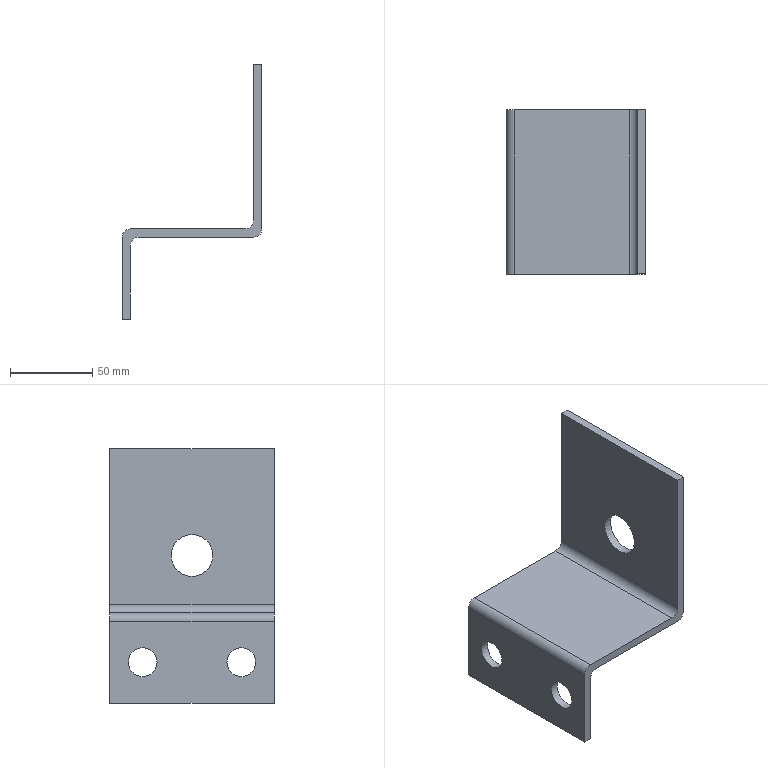Part | NX | features solid 2 | 1 solid | 17 faces | box 85 x 100 x 155 mm | volume 112541 mm3 | plane 10 | cylinder 7 | commonest cylinder face diameters 10 x4 17.5 x2 25.5 x1
STEP:
#1=CARTESIAN_POINT('',(-1095.,-291.25,-600.));
#2=VERTEX_POINT('',#1);
#3=CARTESIAN_POINT('',(-1095.,-300.,-600.));
#4=DIRECTION('',(1.,0.,0.));
#5=DIRECTION('',(0.,1.,0.));
#6=AXIS2_PLACEMENT_3D('',#3,#4,#5);
#7=CIRCLE('',#6,8.75);
#8=EDGE_CURVE('',#2,#2,#7,.T.);
#9=ORIENTED_EDGE('',*,*,#8,.F.);
#10=EDGE_LOOP('',(#9));
#11=FACE_BOUND('',#10,.T.);
#12=CARTESIAN_POINT('',(-1095.,-231.25,-600.));
#13=VERTEX_POINT('',#12);
#14=CARTESIAN_POINT('',(-1095.,-240.,-600.));
#15=DIRECTION('',(1.,0.,0.));
#16=DIRECTION('',(0.,1.,0.));
#17=AXIS2_PLACEMENT_3D('',#14,#15,#16);
#18=CIRCLE('',#17,8.75);
#19=EDGE_CURVE('',#13,#13,#18,.T.);
#20=ORIENTED_EDGE('',*,*,#19,.F.);
#21=EDGE_LOOP('',(#20));
#22=FACE_BOUND('',#21,.T.);
#23=CARTESIAN_POINT('',(-1095.,-220.,-580.));
#24=VERTEX_POINT('',#23);
#25=CARTESIAN_POINT('',(-1095.,-220.,-625.));
#26=VERTEX_POINT('',#25);
#27=CARTESIAN_POINT('',(-1095.,-220.,-570.));
#28=DIRECTION('',(0.,0.,1.));
#29=VECTOR('',#28,1000.);
#30=LINE('',#27,#29);
#31=EDGE_CURVE('',#24,#26,#30,.F.);
#32=ORIENTED_EDGE('',*,*,#31,.F.);
#33=CARTESIAN_POINT('',(-1095.,-320.,-580.));
#34=VERTEX_POINT('',#33);
#35=CARTESIAN_POINT('',(-1095.,-220.,-580.));
#36=DIRECTION('',(0.,-1.,0.));
#37=VECTOR('',#36,1000.);
#38=LINE('',#35,#37);
#39=EDGE_CURVE('',#24,#34,#38,.T.);
#40=ORIENTED_EDGE('',*,*,#39,.T.);
#41=CARTESIAN_POINT('',(-1095.,-320.,-625.));
#42=VERTEX_POINT('',#41);
#43=CARTESIAN_POINT('',(-1095.,-320.,-570.));
#44=DIRECTION('',(0.,0.,1.));
#45=VECTOR('',#44,1000.);
#46=LINE('',#43,#45);
#47=EDGE_CURVE('',#34,#42,#46,.F.);
#48=ORIENTED_EDGE('',*,*,#47,.T.);
#49=CARTESIAN_POINT('',(-1095.,-220.,-625.));
#50=DIRECTION('',(0.,1.,0.));
#51=VECTOR('',#50,1000.);
#52=LINE('',#49,#51);
#53=EDGE_CURVE('',#26,#42,#52,.F.);
#54=ORIENTED_EDGE('',*,*,#53,.F.);
#55=EDGE_LOOP('',(#32,#40,#48,#54));
#56=FACE_BOUND('',#55,.T.);
#57=CARTESIAN_POINT('',(-1095.,-220.,-570.));
#58=DIRECTION('',(1.,0.,0.));
#59=DIRECTION('',(0.,1.,0.));
#60=AXIS2_PLACEMENT_3D('',#57,#58,#59);
#61=PLANE('',#60);
#62=ADVANCED_FACE('',(#11,#22,#56),#61,.T.);
#63=CARTESIAN_POINT('',(-1095.,-220.,-570.));
#64=VERTEX_POINT('',#63);
#65=CARTESIAN_POINT('',(-1025.,-220.,-570.));
#66=VERTEX_POINT('',#65);
#67=CARTESIAN_POINT('',(-1100.,-220.,-570.));
#68=DIRECTION('',(1.,0.,0.));
#69=VECTOR('',#68,1000.);
#70=LINE('',#67,#69);
#71=EDGE_CURVE('',#64,#66,#70,.T.);
#72=ORIENTED_EDGE('',*,*,#71,.F.);
#73=CARTESIAN_POINT('',(-1095.,-320.,-570.));
#74=VERTEX_POINT('',#73);
#75=CARTESIAN_POINT('',(-1095.,-320.,-570.));
#76=DIRECTION('',(0.,-1.,0.));
#77=VECTOR('',#76,1000.);
#78=LINE('',#75,#77);
#79=EDGE_CURVE('',#64,#74,#78,.T.);
#80=ORIENTED_EDGE('',*,*,#79,.T.);
#81=CARTESIAN_POINT('',(-1025.,-320.,-570.));
#82=VERTEX_POINT('',#81);
#83=CARTESIAN_POINT('',(-1100.,-320.,-570.));
#84=DIRECTION('',(1.,0.,0.));
#85=VECTOR('',#84,1000.);
#86=LINE('',#83,#85);
#87=EDGE_CURVE('',#74,#82,#86,.T.);
#88=ORIENTED_EDGE('',*,*,#87,.T.);
#89=CARTESIAN_POINT('',(-1025.,-220.,-570.));
#90=DIRECTION('',(0.,-1.,0.));
#91=VECTOR('',#90,1000.);
#92=LINE('',#89,#91);
#93=EDGE_CURVE('',#82,#66,#92,.F.);
#94=ORIENTED_EDGE('',*,*,#93,.T.);
#95=EDGE_LOOP('',(#72,#80,#88,#94));
#96=FACE_BOUND('',#95,.T.);
#97=CARTESIAN_POINT('',(-1100.,-220.,-570.));
#98=DIRECTION('',(0.,0.,1.));
#99=DIRECTION('',(0.,-1.,0.));
#100=AXIS2_PLACEMENT_3D('',#97,#98,#99);
#101=PLANE('',#100);
#102=ADVANCED_FACE('',(#96),#101,.T.);
#103=ORIENTED_EDGE('',*,*,#87,.F.);
#104=CARTESIAN_POINT('',(-1100.,-320.,-575.));
#105=VERTEX_POINT('',#104);
#106=CARTESIAN_POINT('',(-1095.,-320.,-575.));
#107=DIRECTION('',(0.,-1.,0.));
#108=DIRECTION('',(1.,0.,0.));
#109=AXIS2_PLACEMENT_3D('',#106,#107,#108);
#110=CIRCLE('',#109,5.);
#111=EDGE_CURVE('',#74,#105,#110,.T.);
#112=ORIENTED_EDGE('',*,*,#111,.T.);
#113=CARTESIAN_POINT('',(-1100.,-320.,-625.));
#114=VERTEX_POINT('',#113);
#115=CARTESIAN_POINT('',(-1100.,-320.,-570.));
#116=DIRECTION('',(0.,0.,-1.));
#117=VECTOR('',#116,1000.);
#118=LINE('',#115,#117);
#119=EDGE_CURVE('',#105,#114,#118,.T.);
#120=ORIENTED_EDGE('',*,*,#119,.T.);
#121=CARTESIAN_POINT('',(-1100.,-320.,-625.));
#122=DIRECTION('',(-1.,0.,0.));
#123=VECTOR('',#122,1000.);
#124=LINE('',#121,#123);
#125=EDGE_CURVE('',#114,#42,#124,.F.);
#126=ORIENTED_EDGE('',*,*,#125,.T.);
#127=ORIENTED_EDGE('',*,*,#47,.F.);
#128=CARTESIAN_POINT('',(-1090.,-320.,-575.));
#129=VERTEX_POINT('',#128);
#130=CARTESIAN_POINT('',(-1090.,-320.,-580.));
#131=DIRECTION('',(0.,-1.,0.));
#132=DIRECTION('',(1.,0.,0.));
#133=AXIS2_PLACEMENT_3D('',#130,#131,#132);
#134=CIRCLE('',#133,5.);
#135=EDGE_CURVE('',#34,#129,#134,.F.);
#136=ORIENTED_EDGE('',*,*,#135,.T.);
#137=CARTESIAN_POINT('',(-1020.,-320.,-575.));
#138=VERTEX_POINT('',#137);
#139=CARTESIAN_POINT('',(-1015.,-320.,-575.));
#140=DIRECTION('',(-1.,0.,0.));
#141=VECTOR('',#140,1000.);
#142=LINE('',#139,#141);
#143=EDGE_CURVE('',#138,#129,#142,.T.);
#144=ORIENTED_EDGE('',*,*,#143,.F.);
#145=CARTESIAN_POINT('',(-1015.,-320.,-570.));
#146=VERTEX_POINT('',#145);
#147=CARTESIAN_POINT('',(-1020.,-320.,-570.));
#148=DIRECTION('',(0.,-1.,0.));
#149=DIRECTION('',(1.,0.,0.));
#150=AXIS2_PLACEMENT_3D('',#147,#148,#149);
#151=CIRCLE('',#150,5.);
#152=EDGE_CURVE('',#138,#146,#151,.T.);
#153=ORIENTED_EDGE('',*,*,#152,.T.);
#154=CARTESIAN_POINT('',(-1015.,-320.,-470.));
#155=VERTEX_POINT('',#154);
#156=CARTESIAN_POINT('',(-1015.,-320.,-575.));
#157=DIRECTION('',(0.,0.,1.));
#158=VECTOR('',#157,1000.);
#159=LINE('',#156,#158);
#160=EDGE_CURVE('',#146,#155,#159,.T.);
#161=ORIENTED_EDGE('',*,*,#160,.T.);
#162=CARTESIAN_POINT('',(-1020.,-320.,-470.));
#163=VERTEX_POINT('',#162);
#164=CARTESIAN_POINT('',(-1010.,-320.,-470.));
#165=DIRECTION('',(-1.,0.,0.));
#166=VECTOR('',#165,1000.);
#167=LINE('',#164,#166);
#168=EDGE_CURVE('',#155,#163,#167,.T.);
#169=ORIENTED_EDGE('',*,*,#168,.T.);
#170=CARTESIAN_POINT('',(-1020.,-320.,-565.));
#171=VERTEX_POINT('',#170);
#172=CARTESIAN_POINT('',(-1020.,-320.,-575.));
#173=DIRECTION('',(0.,0.,1.));
#174=VECTOR('',#173,1000.);
#175=LINE('',#172,#174);
#176=EDGE_CURVE('',#171,#163,#175,.T.);
#177=ORIENTED_EDGE('',*,*,#176,.F.);
#178=CARTESIAN_POINT('',(-1025.,-320.,-565.));
#179=DIRECTION('',(0.,-1.,0.));
#180=DIRECTION('',(1.,0.,0.));
#181=AXIS2_PLACEMENT_3D('',#178,#179,#180);
#182=CIRCLE('',#181,5.);
#183=EDGE_CURVE('',#171,#82,#182,.F.);
#184=ORIENTED_EDGE('',*,*,#183,.T.);
#185=EDGE_LOOP('',(#103,#112,#120,#126,#127,#136,#144,#153,#161,#169,#177,#184));
#186=FACE_BOUND('',#185,.T.);
#187=CARTESIAN_POINT('',(-1100.,-320.,-570.));
#188=DIRECTION('',(0.,-1.,0.));
#189=DIRECTION('',(0.,0.,-1.));
#190=AXIS2_PLACEMENT_3D('',#187,#188,#189);
#191=PLANE('',#190);
#192=ADVANCED_FACE('',(#186),#191,.T.);
#193=ORIENTED_EDGE('',*,*,#125,.F.);
#194=CARTESIAN_POINT('',(-1100.,-220.,-625.));
#195=VERTEX_POINT('',#194);
#196=CARTESIAN_POINT('',(-1100.,-220.,-625.));
#197=DIRECTION('',(0.,1.,0.));
#198=VECTOR('',#197,1000.);
#199=LINE('',#196,#198);
#200=EDGE_CURVE('',#195,#114,#199,.F.);
#201=ORIENTED_EDGE('',*,*,#200,.F.);
#202=CARTESIAN_POINT('',(-1100.,-220.,-625.));
#203=DIRECTION('',(1.,0.,0.));
#204=VECTOR('',#203,1000.);
#205=LINE('',#202,#204);
#206=EDGE_CURVE('',#195,#26,#205,.T.);
#207=ORIENTED_EDGE('',*,*,#206,.T.);
#208=ORIENTED_EDGE('',*,*,#53,.T.);
#209=EDGE_LOOP('',(#193,#201,#207,#208));
#210=FACE_BOUND('',#209,.T.);
#211=CARTESIAN_POINT('',(-1100.,-220.,-625.));
#212=DIRECTION('',(0.,0.,1.));
#213=DIRECTION('',(0.,-1.,0.));
#214=AXIS2_PLACEMENT_3D('',#211,#212,#213);
#215=PLANE('',#214);
#216=ADVANCED_FACE('',(#210),#215,.F.);
#217=CARTESIAN_POINT('',(-1100.,-220.,-575.));
#218=VERTEX_POINT('',#217);
#219=CARTESIAN_POINT('',(-1100.,-220.,-570.));
#220=DIRECTION('',(0.,0.,-1.));
#221=VECTOR('',#220,1000.);
#222=LINE('',#219,#221);
#223=EDGE_CURVE('',#218,#195,#222,.T.);
#224=ORIENTED_EDGE('',*,*,#223,.F.);
#225=CARTESIAN_POINT('',(-1095.,-220.,-575.));
#226=DIRECTION('',(0.,-1.,0.));
#227=DIRECTION('',(1.,0.,0.));
#228=AXIS2_PLACEMENT_3D('',#225,#226,#227);
#229=CIRCLE('',#228,5.);
#230=EDGE_CURVE('',#218,#64,#229,.F.);
#231=ORIENTED_EDGE('',*,*,#230,.T.);
#232=ORIENTED_EDGE('',*,*,#71,.T.);
#233=CARTESIAN_POINT('',(-1020.,-220.,-565.));
#234=VERTEX_POINT('',#233);
#235=CARTESIAN_POINT('',(-1025.,-220.,-565.));
#236=DIRECTION('',(0.,-1.,0.));
#237=DIRECTION('',(1.,0.,0.));
#238=AXIS2_PLACEMENT_3D('',#235,#236,#237);
#239=CIRCLE('',#238,5.);
#240=EDGE_CURVE('',#66,#234,#239,.T.);
#241=ORIENTED_EDGE('',*,*,#240,.T.);
#242=CARTESIAN_POINT('',(-1020.,-220.,-470.));
#243=VERTEX_POINT('',#242);
#244=CARTESIAN_POINT('',(-1020.,-220.,-570.));
#245=DIRECTION('',(0.,0.,-1.));
#246=VECTOR('',#245,1000.);
#247=LINE('',#244,#246);
#248=EDGE_CURVE('',#234,#243,#247,.F.);
#249=ORIENTED_EDGE('',*,*,#248,.T.);
#250=CARTESIAN_POINT('',(-1015.,-220.,-470.));
#251=VERTEX_POINT('',#250);
#252=CARTESIAN_POINT('',(-1015.,-220.,-470.));
#253=DIRECTION('',(1.,0.,0.));
#254=VECTOR('',#253,1000.);
#255=LINE('',#252,#254);
#256=EDGE_CURVE('',#251,#243,#255,.F.);
#257=ORIENTED_EDGE('',*,*,#256,.F.);
#258=CARTESIAN_POINT('',(-1015.,-220.,-570.));
#259=VERTEX_POINT('',#258);
#260=CARTESIAN_POINT('',(-1015.,-220.,-570.));
#261=DIRECTION('',(0.,0.,-1.));
#262=VECTOR('',#261,1000.);
#263=LINE('',#260,#262);
#264=EDGE_CURVE('',#259,#251,#263,.F.);
#265=ORIENTED_EDGE('',*,*,#264,.F.);
#266=CARTESIAN_POINT('',(-1020.,-220.,-575.));
#267=VERTEX_POINT('',#266);
#268=CARTESIAN_POINT('',(-1020.,-220.,-570.));
#269=DIRECTION('',(0.,-1.,0.));
#270=DIRECTION('',(1.,0.,0.));
#271=AXIS2_PLACEMENT_3D('',#268,#269,#270);
#272=CIRCLE('',#271,5.);
#273=EDGE_CURVE('',#259,#267,#272,.F.);
#274=ORIENTED_EDGE('',*,*,#273,.T.);
#275=CARTESIAN_POINT('',(-1090.,-220.,-575.));
#276=VERTEX_POINT('',#275);
#277=CARTESIAN_POINT('',(-1015.,-220.,-575.));
#278=DIRECTION('',(-1.,0.,0.));
#279=VECTOR('',#278,1000.);
#280=LINE('',#277,#279);
#281=EDGE_CURVE('',#267,#276,#280,.T.);
#282=ORIENTED_EDGE('',*,*,#281,.T.);
#283=CARTESIAN_POINT('',(-1090.,-220.,-580.));
#284=DIRECTION('',(0.,-1.,0.));
#285=DIRECTION('',(1.,0.,0.));
#286=AXIS2_PLACEMENT_3D('',#283,#284,#285);
#287=CIRCLE('',#286,5.);
#288=EDGE_CURVE('',#276,#24,#287,.T.);
#289=ORIENTED_EDGE('',*,*,#288,.T.);
#290=ORIENTED_EDGE('',*,*,#31,.T.);
#291=ORIENTED_EDGE('',*,*,#206,.F.);
#292=EDGE_LOOP('',(#224,#231,#232,#241,#249,#257,#265,#274,#282,#289,#290,#291));
#293=FACE_BOUND('',#292,.T.);
#294=CARTESIAN_POINT('',(-1100.,-220.,-570.));
#295=DIRECTION('',(0.,-1.,0.));
#296=DIRECTION('',(0.,0.,-1.));
#297=AXIS2_PLACEMENT_3D('',#294,#295,#296);
#298=PLANE('',#297);
#299=ADVANCED_FACE('',(#293),#298,.F.);
#300=CARTESIAN_POINT('',(-1100.,-291.25,-600.));
#301=VERTEX_POINT('',#300);
#302=CARTESIAN_POINT('',(-1100.,-300.,-600.));
#303=DIRECTION('',(1.,0.,0.));
#304=DIRECTION('',(0.,1.,0.));
#305=AXIS2_PLACEMENT_3D('',#302,#303,#304);
#306=CIRCLE('',#305,8.75);
#307=EDGE_CURVE('',#301,#301,#306,.T.);
#308=ORIENTED_EDGE('',*,*,#307,.T.);
#309=EDGE_LOOP('',(#308));
#310=FACE_BOUND('',#309,.T.);
#311=CARTESIAN_POINT('',(-1100.,-231.25,-600.));
#312=VERTEX_POINT('',#311);
#313=CARTESIAN_POINT('',(-1100.,-240.,-600.));
#314=DIRECTION('',(1.,0.,0.));
#315=DIRECTION('',(0.,1.,0.));
#316=AXIS2_PLACEMENT_3D('',#313,#314,#315);
#317=CIRCLE('',#316,8.75);
#318=EDGE_CURVE('',#312,#312,#317,.T.);
#319=ORIENTED_EDGE('',*,*,#318,.T.);
#320=EDGE_LOOP('',(#319));
#321=FACE_BOUND('',#320,.T.);
#322=ORIENTED_EDGE('',*,*,#119,.F.);
#323=CARTESIAN_POINT('',(-1100.,-220.,-575.));
#324=DIRECTION('',(0.,-1.,0.));
#325=VECTOR('',#324,1000.);
#326=LINE('',#323,#325);
#327=EDGE_CURVE('',#105,#218,#326,.F.);
#328=ORIENTED_EDGE('',*,*,#327,.T.);
#329=ORIENTED_EDGE('',*,*,#223,.T.);
#330=ORIENTED_EDGE('',*,*,#200,.T.);
#331=EDGE_LOOP('',(#322,#328,#329,#330));
#332=FACE_BOUND('',#331,.T.);
#333=CARTESIAN_POINT('',(-1100.,-220.,-570.));
#334=DIRECTION('',(1.,0.,0.));
#335=DIRECTION('',(0.,1.,0.));
#336=AXIS2_PLACEMENT_3D('',#333,#334,#335);
#337=PLANE('',#336);
#338=ADVANCED_FACE('',(#310,#321,#332),#337,.F.);
#339=CARTESIAN_POINT('',(-1015.,-270.,-522.25));
#340=VERTEX_POINT('',#339);
#341=CARTESIAN_POINT('',(-1015.,-270.,-535.));
#342=DIRECTION('',(-1.,0.,0.));
#343=DIRECTION('',(0.,0.,1.));
#344=AXIS2_PLACEMENT_3D('',#341,#342,#343);
#345=CIRCLE('',#344,12.75);
#346=EDGE_CURVE('',#340,#340,#345,.T.);
#347=ORIENTED_EDGE('',*,*,#346,.T.);
#348=EDGE_LOOP('',(#347));
#349=FACE_BOUND('',#348,.T.);
#350=ORIENTED_EDGE('',*,*,#160,.F.);
#351=CARTESIAN_POINT('',(-1015.,-210.,-570.));
#352=DIRECTION('',(0.,-1.,0.));
#353=VECTOR('',#352,1000.);
#354=LINE('',#351,#353);
#355=EDGE_CURVE('',#146,#259,#354,.F.);
#356=ORIENTED_EDGE('',*,*,#355,.T.);
#357=ORIENTED_EDGE('',*,*,#264,.T.);
#358=CARTESIAN_POINT('',(-1015.,-210.,-470.));
#359=DIRECTION('',(0.,-1.,0.));
#360=VECTOR('',#359,1000.);
#361=LINE('',#358,#360);
#362=EDGE_CURVE('',#251,#155,#361,.T.);
#363=ORIENTED_EDGE('',*,*,#362,.T.);
#364=EDGE_LOOP('',(#350,#356,#357,#363));
#365=FACE_BOUND('',#364,.T.);
#366=CARTESIAN_POINT('',(-1015.,-210.,-575.));
#367=DIRECTION('',(-1.,0.,0.));
#368=DIRECTION('',(0.,0.,1.));
#369=AXIS2_PLACEMENT_3D('',#366,#367,#368);
#370=PLANE('',#369);
#371=ADVANCED_FACE('',(#349,#365),#370,.F.);
#372=ORIENTED_EDGE('',*,*,#143,.T.);
#373=CARTESIAN_POINT('',(-1090.,-210.,-575.));
#374=DIRECTION('',(0.,-1.,0.));
#375=VECTOR('',#374,1000.);
#376=LINE('',#373,#375);
#377=EDGE_CURVE('',#129,#276,#376,.F.);
#378=ORIENTED_EDGE('',*,*,#377,.T.);
#379=ORIENTED_EDGE('',*,*,#281,.F.);
#380=CARTESIAN_POINT('',(-1020.,-210.,-575.));
#381=DIRECTION('',(0.,-1.,0.));
#382=VECTOR('',#381,1000.);
#383=LINE('',#380,#382);
#384=EDGE_CURVE('',#267,#138,#383,.T.);
#385=ORIENTED_EDGE('',*,*,#384,.T.);
#386=EDGE_LOOP('',(#372,#378,#379,#385));
#387=FACE_BOUND('',#386,.T.);
#388=CARTESIAN_POINT('',(-1015.,-210.,-575.));
#389=DIRECTION('',(0.,0.,1.));
#390=DIRECTION('',(-1.,0.,0.));
#391=AXIS2_PLACEMENT_3D('',#388,#389,#390);
#392=PLANE('',#391);
#393=ADVANCED_FACE('',(#387),#392,.F.);
#394=ORIENTED_EDGE('',*,*,#168,.F.);
#395=ORIENTED_EDGE('',*,*,#362,.F.);
#396=ORIENTED_EDGE('',*,*,#256,.T.);
#397=CARTESIAN_POINT('',(-1020.,-210.,-470.));
#398=DIRECTION('',(0.,-1.,0.));
#399=VECTOR('',#398,1000.);
#400=LINE('',#397,#399);
#401=EDGE_CURVE('',#243,#163,#400,.T.);
#402=ORIENTED_EDGE('',*,*,#401,.T.);
#403=EDGE_LOOP('',(#394,#395,#396,#402));
#404=FACE_BOUND('',#403,.T.);
#405=CARTESIAN_POINT('',(-1015.,-210.,-470.));
#406=DIRECTION('',(0.,0.,1.));
#407=DIRECTION('',(-1.,0.,0.));
#408=AXIS2_PLACEMENT_3D('',#405,#406,#407);
#409=PLANE('',#408);
#410=ADVANCED_FACE('',(#404),#409,.T.);
#411=CARTESIAN_POINT('',(-1020.,-270.,-522.25));
#412=VERTEX_POINT('',#411);
#413=CARTESIAN_POINT('',(-1020.,-270.,-535.));
#414=DIRECTION('',(-1.,0.,0.));
#415=DIRECTION('',(0.,0.,1.));
#416=AXIS2_PLACEMENT_3D('',#413,#414,#415);
#417=CIRCLE('',#416,12.75);
#418=EDGE_CURVE('',#412,#412,#417,.T.);
#419=ORIENTED_EDGE('',*,*,#418,.F.);
#420=EDGE_LOOP('',(#419));
#421=FACE_BOUND('',#420,.T.);
#422=ORIENTED_EDGE('',*,*,#248,.F.);
#423=CARTESIAN_POINT('',(-1020.,-320.,-565.));
#424=DIRECTION('',(0.,-1.,0.));
#425=VECTOR('',#424,1000.);
#426=LINE('',#423,#425);
#427=EDGE_CURVE('',#234,#171,#426,.T.);
#428=ORIENTED_EDGE('',*,*,#427,.T.);
#429=ORIENTED_EDGE('',*,*,#176,.T.);
#430=ORIENTED_EDGE('',*,*,#401,.F.);
#431=EDGE_LOOP('',(#422,#428,#429,#430));
#432=FACE_BOUND('',#431,.T.);
#433=CARTESIAN_POINT('',(-1020.,-220.,-575.));
#434=DIRECTION('',(-1.,0.,0.));
#435=DIRECTION('',(0.,0.,1.));
#436=AXIS2_PLACEMENT_3D('',#433,#434,#435);
#437=PLANE('',#436);
#438=ADVANCED_FACE('',(#421,#432),#437,.T.);
#439=ORIENTED_EDGE('',*,*,#418,.T.);
#440=EDGE_LOOP('',(#439));
#441=FACE_BOUND('',#440,.T.);
#442=ORIENTED_EDGE('',*,*,#346,.F.);
#443=EDGE_LOOP('',(#442));
#444=FACE_BOUND('',#443,.T.);
#445=CARTESIAN_POINT('',(-1021.6,-270.,-535.));
#446=DIRECTION('',(1.,0.,0.));
#447=DIRECTION('',(0.,0.,-1.));
#448=AXIS2_PLACEMENT_3D('',#445,#446,#447);
#449=CYLINDRICAL_SURFACE('',#448,12.75);
#450=ADVANCED_FACE('',(#441,#444),#449,.F.);
#451=ORIENTED_EDGE('',*,*,#230,.F.);
#452=ORIENTED_EDGE('',*,*,#327,.F.);
#453=ORIENTED_EDGE('',*,*,#111,.F.);
#454=ORIENTED_EDGE('',*,*,#79,.F.);
#455=EDGE_LOOP('',(#451,#452,#453,#454));
#456=FACE_BOUND('',#455,.T.);
#457=CARTESIAN_POINT('',(-1095.,-220.,-575.));
#458=DIRECTION('',(0.,1.,0.));
#459=DIRECTION('',(-1.,0.,0.));
#460=AXIS2_PLACEMENT_3D('',#457,#458,#459);
#461=CYLINDRICAL_SURFACE('',#460,5.);
#462=ADVANCED_FACE('',(#456),#461,.T.);
#463=ORIENTED_EDGE('',*,*,#288,.F.);
#464=ORIENTED_EDGE('',*,*,#377,.F.);
#465=ORIENTED_EDGE('',*,*,#135,.F.);
#466=ORIENTED_EDGE('',*,*,#39,.F.);
#467=EDGE_LOOP('',(#463,#464,#465,#466));
#468=FACE_BOUND('',#467,.T.);
#469=CARTESIAN_POINT('',(-1090.,-220.,-580.));
#470=DIRECTION('',(0.,-1.,0.));
#471=DIRECTION('',(1.,0.,0.));
#472=AXIS2_PLACEMENT_3D('',#469,#470,#471);
#473=CYLINDRICAL_SURFACE('',#472,5.);
#474=ADVANCED_FACE('',(#468),#473,.F.);
#475=ORIENTED_EDGE('',*,*,#273,.F.);
#476=ORIENTED_EDGE('',*,*,#355,.F.);
#477=ORIENTED_EDGE('',*,*,#152,.F.);
#478=ORIENTED_EDGE('',*,*,#384,.F.);
#479=EDGE_LOOP('',(#475,#476,#477,#478));
#480=FACE_BOUND('',#479,.T.);
#481=CARTESIAN_POINT('',(-1020.,-210.,-570.));
#482=DIRECTION('',(0.,-1.,0.));
#483=DIRECTION('',(0.,0.,-1.));
#484=AXIS2_PLACEMENT_3D('',#481,#482,#483);
#485=CYLINDRICAL_SURFACE('',#484,5.);
#486=ADVANCED_FACE('',(#480),#485,.T.);
#487=ORIENTED_EDGE('',*,*,#240,.F.);
#488=ORIENTED_EDGE('',*,*,#93,.F.);
#489=ORIENTED_EDGE('',*,*,#183,.F.);
#490=ORIENTED_EDGE('',*,*,#427,.F.);
#491=EDGE_LOOP('',(#487,#488,#489,#490));
#492=FACE_BOUND('',#491,.T.);
#493=CARTESIAN_POINT('',(-1025.,-220.,-565.));
#494=DIRECTION('',(0.,1.,0.));
#495=DIRECTION('',(0.,0.,1.));
#496=AXIS2_PLACEMENT_3D('',#493,#494,#495);
#497=CYLINDRICAL_SURFACE('',#496,5.);
#498=ADVANCED_FACE('',(#492),#497,.F.);
#499=ORIENTED_EDGE('',*,*,#19,.T.);
#500=EDGE_LOOP('',(#499));
#501=FACE_BOUND('',#500,.T.);
#502=ORIENTED_EDGE('',*,*,#318,.F.);
#503=EDGE_LOOP('',(#502));
#504=FACE_BOUND('',#503,.T.);
#505=CARTESIAN_POINT('',(-1100.,-240.,-600.));
#506=DIRECTION('',(1.,0.,0.));
#507=DIRECTION('',(0.,1.,0.));
#508=AXIS2_PLACEMENT_3D('',#505,#506,#507);
#509=CYLINDRICAL_SURFACE('',#508,8.75);
#510=ADVANCED_FACE('',(#501,#504),#509,.F.);
#511=ORIENTED_EDGE('',*,*,#8,.T.);
#512=EDGE_LOOP('',(#511));
#513=FACE_BOUND('',#512,.T.);
#514=ORIENTED_EDGE('',*,*,#307,.F.);
#515=EDGE_LOOP('',(#514));
#516=FACE_BOUND('',#515,.T.);
#517=CARTESIAN_POINT('',(-1100.,-300.,-600.));
#518=DIRECTION('',(1.,0.,0.));
#519=DIRECTION('',(0.,1.,0.));
#520=AXIS2_PLACEMENT_3D('',#517,#518,#519);
#521=CYLINDRICAL_SURFACE('',#520,8.75);
#522=ADVANCED_FACE('',(#513,#516),#521,.F.);
#523=CLOSED_SHELL('',(#62,#102,#192,#216,#299,#338,#371,#393,#410,#438,#450,#462,#474,#486,#498,#510,#522));
#524=MANIFOLD_SOLID_BREP('',#523);
#525=(LENGTH_UNIT()NAMED_UNIT(*)SI_UNIT(.MILLI.,.METRE.));
#526=UNCERTAINTY_MEASURE_WITH_UNIT(LENGTH_MEASURE(0.00001),#525,'','');
#527=(NAMED_UNIT(*)PLANE_ANGLE_UNIT()SI_UNIT($,.RADIAN.));
#528=(NAMED_UNIT(*)SI_UNIT($,.STERADIAN.)SOLID_ANGLE_UNIT());
#529=(GEOMETRIC_REPRESENTATION_CONTEXT(3)GLOBAL_UNCERTAINTY_ASSIGNED_CONTEXT((#526))GLOBAL_UNIT_ASSIGNED_CONTEXT((#525,#527,#528))REPRESENTATION_CONTEXT('',''));
#530=ADVANCED_BREP_SHAPE_REPRESENTATION('',(#524),#529);